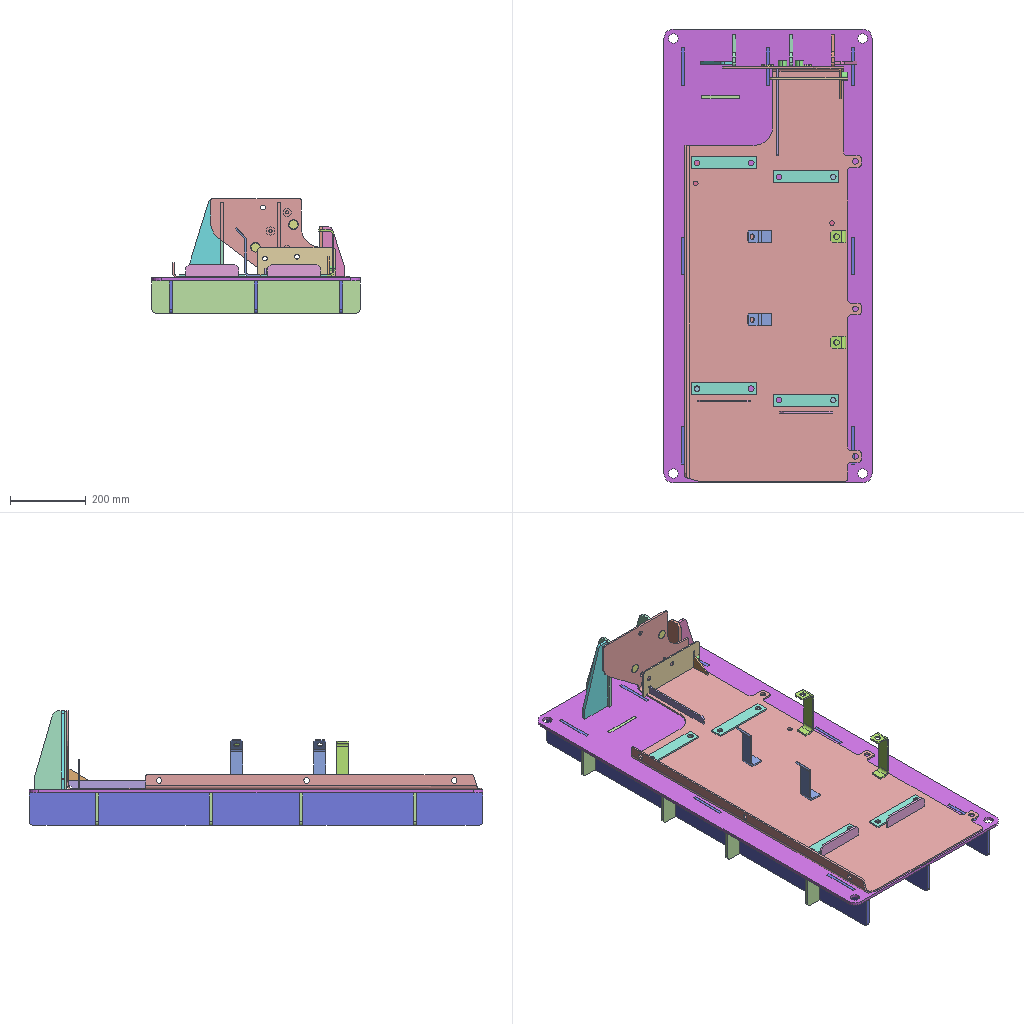Assembly | SolidWorks | 19 different items | 37 placed | box 550 x 1200 x 302 mm
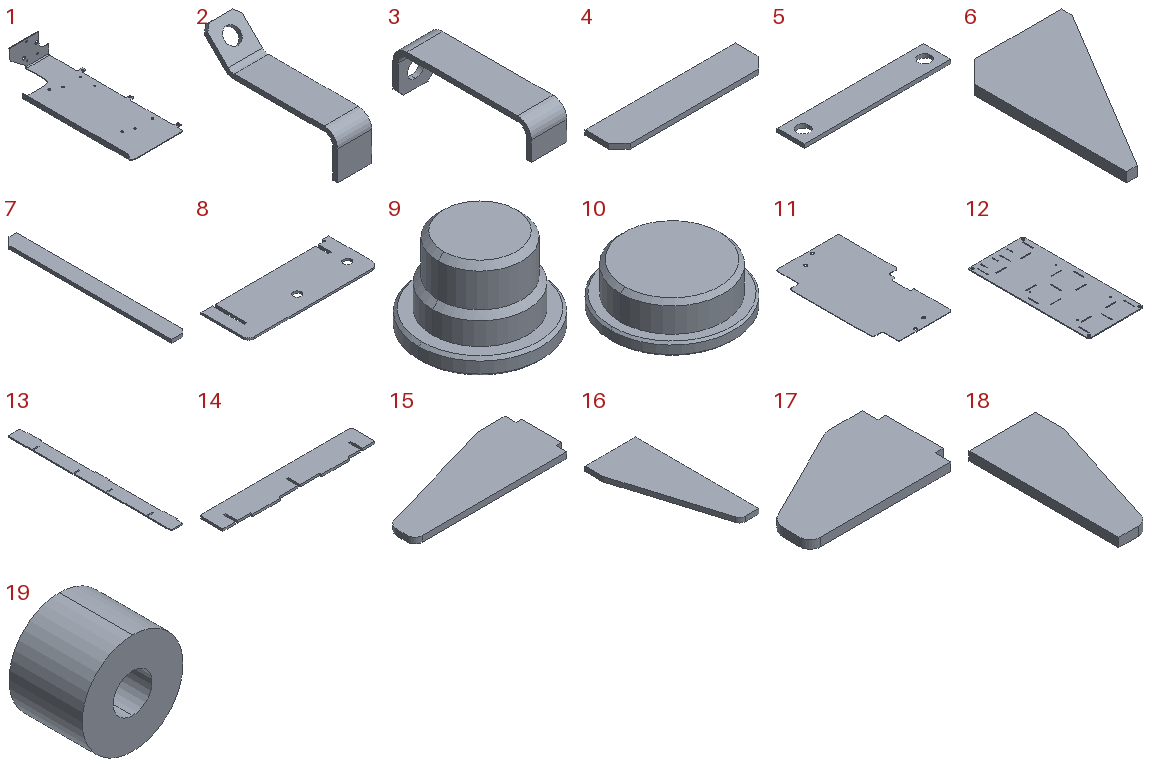Parts list (item | quantity | size | volume | features):
1 | x1 | 466 x 1095 x 209 mm | 2221279 mm3 | features ICE 3, EdgeFlange 2, Fillet 2, FlatPattern 1, Fold 1, SMBaseFlange 1, SheetMetal 1, UnFold 1
2 | x2 | 32 x 128.182 x 65 mm | 23267 mm3 | features Chamfer 1, FlatPattern 1, ICE 1, SMBaseFlange 1, SheetMetal 1
3 | x2 | 32 x 124 x 40 mm | 24465 mm3 | features Chamfer 1, FlatPattern 1, ICE 1, SMBaseFlange 1, SheetMetal 1
4 | x2 | 140 x 32 x 4.5 mm | 19710 mm3 | features FlatPattern 1, SMBaseFlange 1, SheetMetal 1
5 | x4 | 173 x 32 x 4.5 mm | 23322 mm3 | features FlatPattern 1, SMBaseFlange 1, SheetMetal 1
6 | x1 | 50 x 80 x 4.5 mm | 10181 mm3 | features FlatPattern 1, SMBaseFlange 1, SheetMetal 1
7 | x1 | 20 x 230 x 4.5 mm | 20419 mm3 | features FlatPattern 1, SMBaseFlange 1, SheetMetal 1
8 | x1 | 208 x 80 x 3.2 mm | 48747 mm3 | features FlatPattern 1, SMBaseFlange 1, SheetMetal 1
9 | x3 | 22 x 22 x 15 mm | 3447 mm3 | features Chamfer 2, Revolution 1
10 | x2 | 30 x 30 x 10 mm | 5495 mm3 | features Chamfer 2, Revolution 1
11 | x1 | 384.5 x 660 x 2.3 mm | 513423 mm3 | features FlatPattern 1, SMBaseFlange 1, SheetMetal 1
12 | x1 | 550 x 1200 x 8 mm | 5135849 mm3 | features FlatPattern 1, SMBaseFlange 1, SheetMetal 1
13 | x3 | 92.5 x 1200 x 8 mm | 822649 mm3 | features FlatPattern 1, SMBaseFlange 1, SheetMetal 1
14 | x4 | 550 x 92.5 x 8 mm | 377497 mm3 | features FlatPattern 1, SMBaseFlange 1, SheetMetal 1
15 | x2 | 216.5 x 85 x 8 mm | 110253 mm3 | features FlatPattern 1, SMBaseFlange 1, SheetMetal 1
16 | x1 | 85 x 209 x 8 mm | 102657 mm3 | features FlatPattern 1, SMBaseFlange 1, SheetMetal 1
17 | x1 | 142.5 x 85 x 8 mm | 74805 mm3 | features FlatPattern 1, SMBaseFlange 1, SheetMetal 1
18 | x1 | 60 x 135 x 8 mm | 49319 mm3 | features FlatPattern 1, SMBaseFlange 1, SheetMetal 1
19 | x4 | 22 x 16 x 22 mm | 5174 mm3 | features Extrusion 1, HoleWzd 1
Mates (type | each side: item.copy, entity, surface, feature):
Coincident | 1.1 face plane Base-Flange1 | 2.1 face plane Base-Flange1
DistanceDim | 1.1 face plane Edge-Flange1 | 2.1 face plane Base-Flange1
DistanceDim | 1.1 face plane Edge-Flange2 | 2.1 face plane Base-Flange1
Coincident | 1.1 face plane Base-Flange1 | 3.1 face plane Base-Flange1
Coincident | 2.1 face plane Base-Flange1 | 3.1 face plane Base-Flange1
DistanceDim | 1.1 face plane Edge-Flange1 | 3.1 face cylinder Cut-Extrude1
Coincident | 1.1 face plane Base-Flange1 | 4.1 face plane Base-Flange1
DistanceDim | 1.1 face plane Edge-Flange1 | 4.1 face plane Base-Flange1
DistanceDim | 4.1 face plane Base-Flange1 | 1.1 face plane Base-Flange1
Coincident | 1.1 face plane Base-Flange1 | 4.2 face plane Base-Flange1
DistanceDim | 4.2 face plane Base-Flange1 | 4.1 face plane Base-Flange1
DistanceDim | 4.2 face plane Base-Flange1 | 1.1 face plane Edge-Flange1
Coincident | 1.1 face plane Base-Flange1 | 5.1 face plane Base-Flange1
Concentric | 1.1 face cylinder Base-Flange1 | 5.1 face cylinder Base-Flange1 | 2 times
Coincident | 1.1 face plane Base-Flange1 | 5.2 face plane Base-Flange1
Concentric | 1.1 face cylinder Base-Flange1 | 5.2 face cylinder Base-Flange1 | 2 times
Coincident | 1.1 face plane Base-Flange1 | 5.3 face plane Base-Flange1
Concentric | 1.1 face cylinder Base-Flange1 | 5.3 face cylinder Base-Flange1 | 2 times
Coincident | 1.1 face plane Base-Flange1 | 5.4 face plane Base-Flange1
Concentric | 1.1 face cylinder Base-Flange1 | 5.4 face cylinder Base-Flange1 | 2 times
Coincident | 1.1 face plane Base-Flange1 | 6.1 face plane Base-Flange1
Coincident | 1.1 face plane Edge-Flange2 | 6.1 face plane Base-Flange1
DistanceDim | 1.1 face plane Base-Flange1 | 6.1 face plane Base-Flange1
Coincident | 1.1 face plane Base-Flange1 | 7.1 face plane Base-Flange1
Coincident | 1.1 face plane Edge-Flange2 | 7.1 face plane Base-Flange1
DistanceDim | 7.1 face plane Base-Flange1 | 1.1 face plane Cut-Extrude2
Coincident | 1.1 face plane Edge-Flange2 | 19.1 face plane Boss-Extrude1
DistanceDim | 19.1 face cylinder Boss-Extrude1 | 1.1 face plane Base-Flange1
DistanceDim | 19.1 face cylinder Boss-Extrude1 | 1.1 face plane Cut-Extrude2
Coincident | 1.1 face plane Edge-Flange2 | 19.2 face plane Boss-Extrude1
DistanceDim | 19.2 face cylinder Boss-Extrude1 | 1.1 face plane Cut-Extrude2
DistanceDim | 19.1 face cylinder Boss-Extrude1 | 19.2 face cylinder Boss-Extrude1
Coincident | 1.1 face plane Edge-Flange2 | 19.3 face plane Boss-Extrude1
DistanceDim | 19.3 face cylinder Boss-Extrude1 | 1.1 face plane Cut-Extrude2
DistanceDim | 19.3 face cylinder Boss-Extrude1 | 1.1 face plane Base-Flange1
Coincident | 6.1 face plane Base-Flange1 | 19.4 face plane Boss-Extrude1
DistanceDim | 1.1 face plane Edge-Flange2 | 19.4 face cylinder Boss-Extrude1
DistanceDim | 1.1 face plane Base-Flange1 | 19.4 face cylinder Boss-Extrude1
InPlace | 1.1 face plane Base-Flange1 | 11.1 plane
Concentric | 1.1 face cylinder Cut-Extrude2 | 10.1 face cylinder Revolve1
Concentric | 1.1 face cylinder Cut-Extrude2 | 10.2 face cylinder Revolve1
InPlace | 1.1 face plane Base-Flange1 | 12.1 plane
InPlace | 15.1 plane | assembly plane
InPlace | 17.1 plane | assembly plane
InPlace | 13.1 plane | assembly plane
InPlace | 14.1 plane | assembly plane
InPlace | 18.1 plane | assembly plane
InPlace | 16.1 plane | assembly plane
InPlace | 8.1 plane | assembly plane